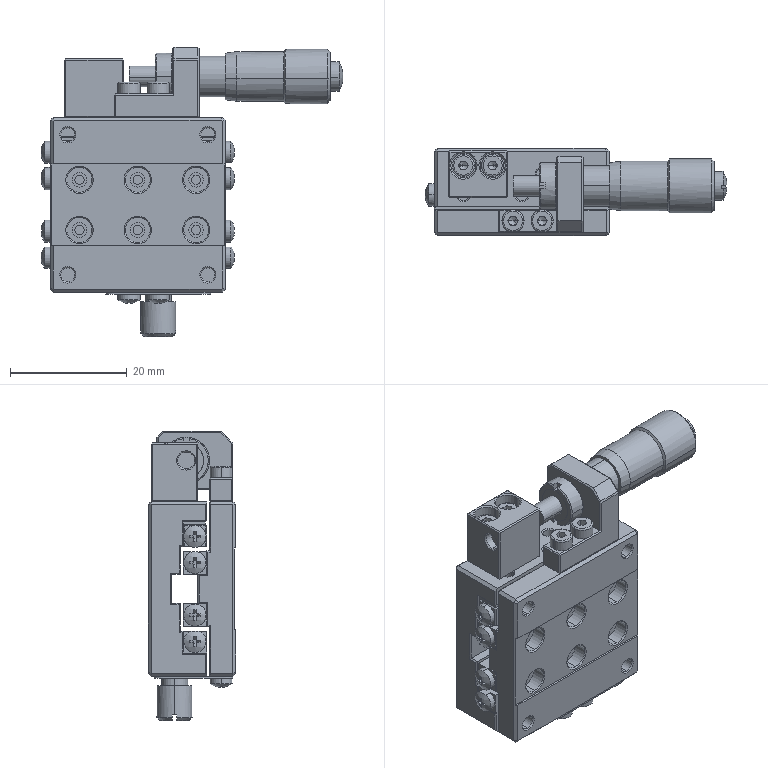Part | SolidWorks | features MBimport 1 | 2 solids | 1011 faces | box 51.773 x 15 x 49.6 mm | volume 14054 mm3 | plane 559 | cylinder 274 | cone 158 | sphere 12 | torus 8 | commonest cylinder face diameters 0.6 x40 1.6 x34 4.3 x32 3.8 x27 2.5 x22 1.5 x18